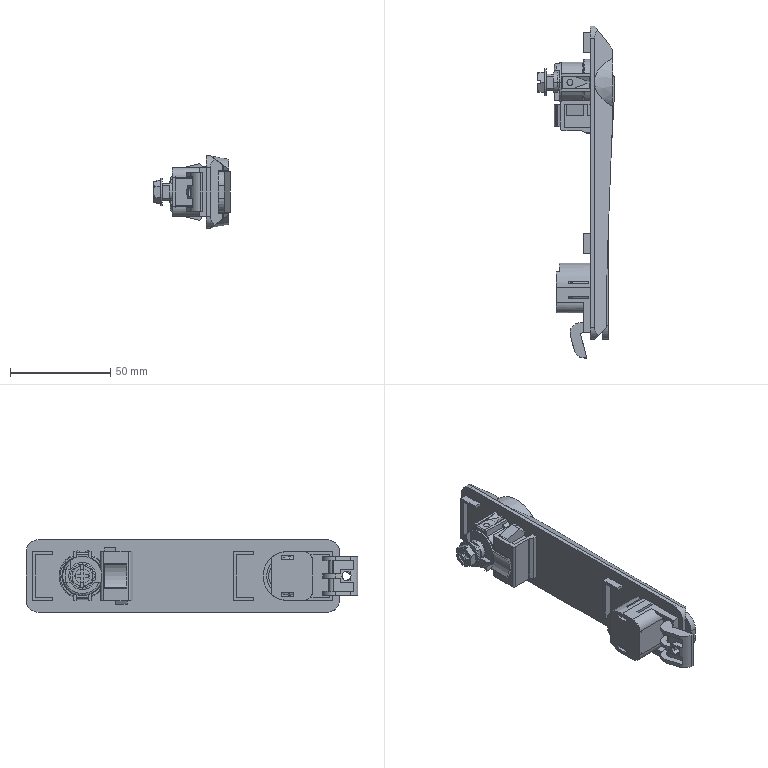Part | SolidWorks | features BaseBody 4 | 4 solids | 621 faces | box 37.95 x 165.2 x 36 mm | volume 54384 mm3 | plane 424 | cylinder 147 | spline 44 | cone 6 | commonest cylinder face diameters 1 x15 10 x12 1000 x12 8 x10 4 x8 12 x7